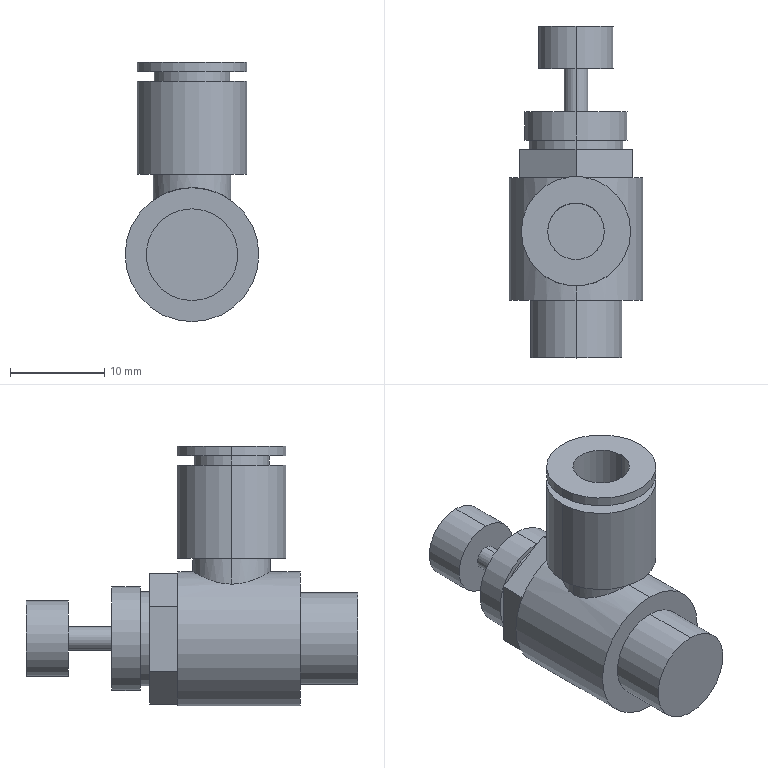Part | STEP file | AS2201F-01-06 | 1 solid | 41 faces | box 14.2 x 35.2 x 27.5 mm | volume 4409 mm3 | cylinder 22 | plane 19 | commonest cylinder face diameters 8 x4 11.6 x4 2.5 x2 6 x2 8.24 x2 9.728 x2